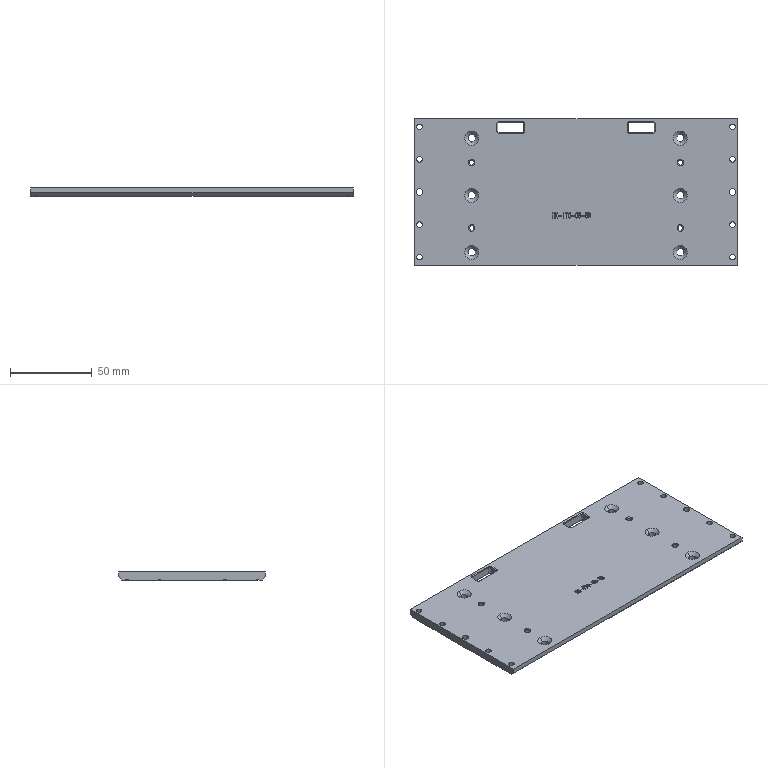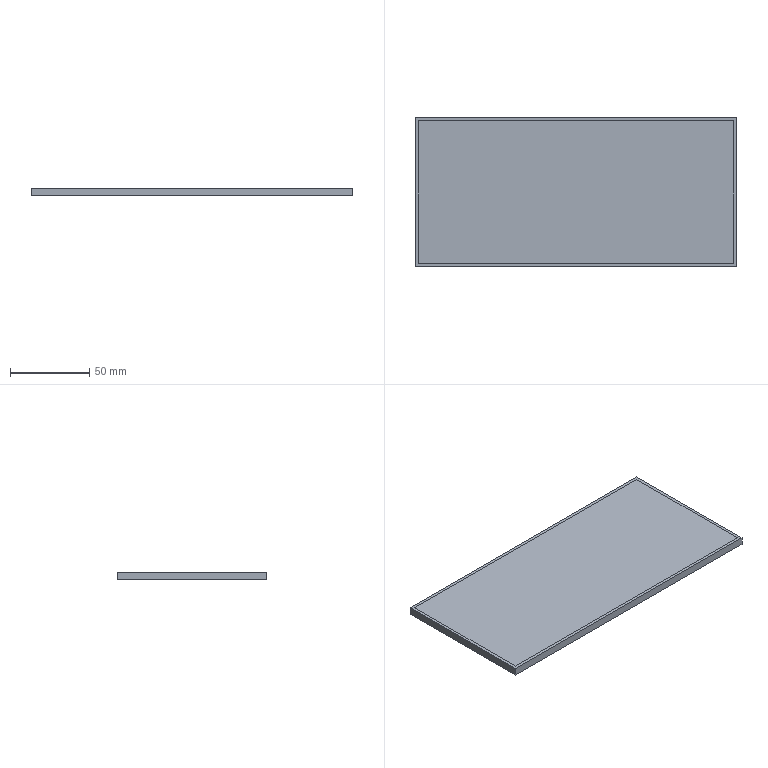CAM job | NX | 3-axis milling, drilling | part box 198 x 90 x 5 mm | stock box 202 x 94 x 5 mm
Tools:
number,name,description,diameter,corner_radius,flute_length,length,flutes
1,D6A45,Milling Tool-5 Parameters,6.0,0.0,50.0,75.0,2
8,4.5ZT,Drilling Tool,4.5,0.0,35.0,50.0,2
16,3.4ZT,Drilling Tool,3.4,0.0,35.0,50.0,2
15,D10,Milling Tool-5 Parameters,10.0,0.0,50.0,75.0,2
14,D10JING,Milling Tool-5 Parameters,10.0,0.0,50.0,75.0,2
11,D4,Milling Tool-5 Parameters,4.0,0.0,50.0,75.0,2
17,D2,Milling Tool-5 Parameters,2.0,0.0,50.0,75.0,2
Operations:
program,operation,operation_type,tool,method,geometry_group,spindle_rpm,surface_speed,feed_per_tooth,feed_cut,feed_plunge,cut_length_mm,path_length_mm,cut_time_min,machine_time_min
1,DRILLING,Operation,D6A45,METHOD,A,5000.0,94.0,0.035,350.0,0.0,11.0,277.023,0.0314,0.058
1,DRILLING_COPY,Operation,D6A45,METHOD,A,5000.0,94.0,0.035,350.0,0.0,20.0,323.363,0.0571,0.0875
1,DRILLING_COPY_COPY,Operation,D6A45,METHOD,A,5000.0,94.0,0.035,350.0,0.0,74.9,743.028,0.214,0.2808
1,DRILLING_COPY_1,Operation,4.5ZT,METHOD,A,2000.0,40.0,0.075,300.0,0.0,65.112,473.772,0.217,0.2579
1,DRILLING_COPY_1_COPY,Operation,3.4ZT,METHOD,A,2000.0,21.0,0.05,200.0,0.0,76.172,586.486,0.3809,0.4319
1,ZLEVEL_PROFILE_COPY_1_COPY,ZLevelMilling,D10,METHOD,A,9500.0,298.0,0.1579,3000.0,1000.0,5512.98,5574.38,1.864,1.87
1,FLOOR_WALL,VolumeBased25DMillingOperation,D10,METHOD,A,9500.0,298.0,0.1579,3000.0,1000.0,4207.035,4848.147,1.779,1.843
1,FLOOR_WALL_COPY,VolumeBased25DMillingOperation,D10JING,METHOD,A,9500.0,298.0,0.0789,1500.0,1000.0,2122.175,2742.784,1.421,1.483
1,ZLEVEL_PROFILE_COPY_1_COPY_COPY,ZLevelMilling,D4,METHOD,A,9500.0,119.0,0.1053,2000.0,1000.0,881.333,1080.405,0.4767,0.4966
1,ZLEVEL_PROFILE_COPY_1_COPY_COPY_COPY,ZLevelMilling,D2,METHOD,A,9500.0,59.0,0.0579,1100.0,1000.0,681.695,1621.511,0.6298,0.7238
1,HOLE_MILLING,CylinderMilling,D2,METHOD,A,9500.0,59.0,0.0579,1100.0,100.0,816.15,1483.413,0.742,0.8087
1,ZLEVEL_PROFILE_COPY_1_COPY_COPY_COPY_1,ZLevelMilling,D6A45,METHOD,A,9500.0,179.0,0.0684,1300.0,1000.0,936.666,1809.604,0.7875,0.8748
1,PLANAR_MILL_COPY_COPY_COPY_COPY_COPY,PlanarMilling,D6A45,METHOD,A,9500.0,179.0,0.0658,1250.0,100.0,1440.349,2200.342,1.152,1.228
1,PLANAR_MILL_COPY_COPY_COPY_COPY_COPY_COPY,PlanarMilling,D6A45,METHOD,A,9500.0,179.0,0.0658,1250.0,100.0,1218.566,2483.505,0.9749,1.101
1,刀补17,CylinderMilling,D2,METHOD,A,9500.0,59.0,0.0579,1100.0,100.0,107.572,774.835,0.0978,0.1645
1,ZLEVEL_PROFILE_COPY_1_COPY_COPY_1,ZLevelMilling,D10JING,METHOD,A,9500.0,298.0,0.0632,1200.0,1000.0,3044.38,3111.805,2.538,2.544
2,ZLEVEL_PROFILE_COPY_1_COPY_COPY_COPY_1_COPY,ZLevelMilling,D6A45,METHOD,B,9500.0,179.0,0.0684,1300.0,1000.0,1070.018,1695.537,0.8722,0.9348
2,PLANAR_MILL_COPY_COPY_COPY_COPY_COPY_COPY_1,PlanarMilling,D6A45,METHOD,B,9500.0,179.0,0.0658,1250.0,100.0,112.544,695.036,0.09,0.1483
2,PLANAR_MILL_COPY_COPY_COPY_COPY_COPY_COPY_1_COPY,PlanarMilling,D6A45,METHOD,B,9500.0,179.0,0.0658,1250.0,100.0,950.325,2802.882,0.7603,0.9455